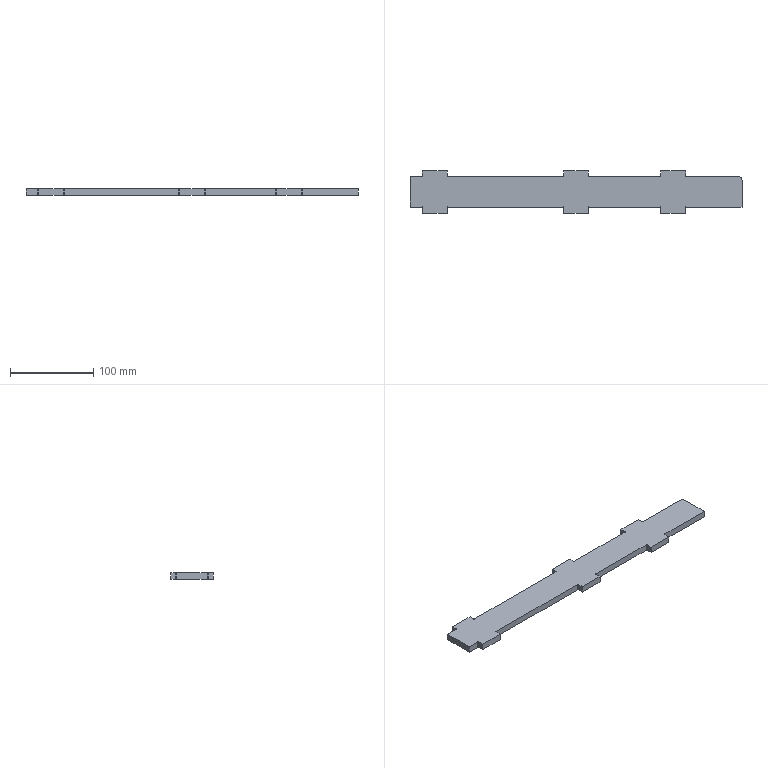Part | SolidWorks | features Fillet 2, FlatPattern 1, ICE 1, SMBaseFlange 1, SheetMetal 1 | 1 solid | 73 faces | box 400 x 51.5 x 8 mm | volume 128767 mm3 | cylinder 43 | plane 30 | commonest cylinder face diameters 2 x24 1 x18 10 x1